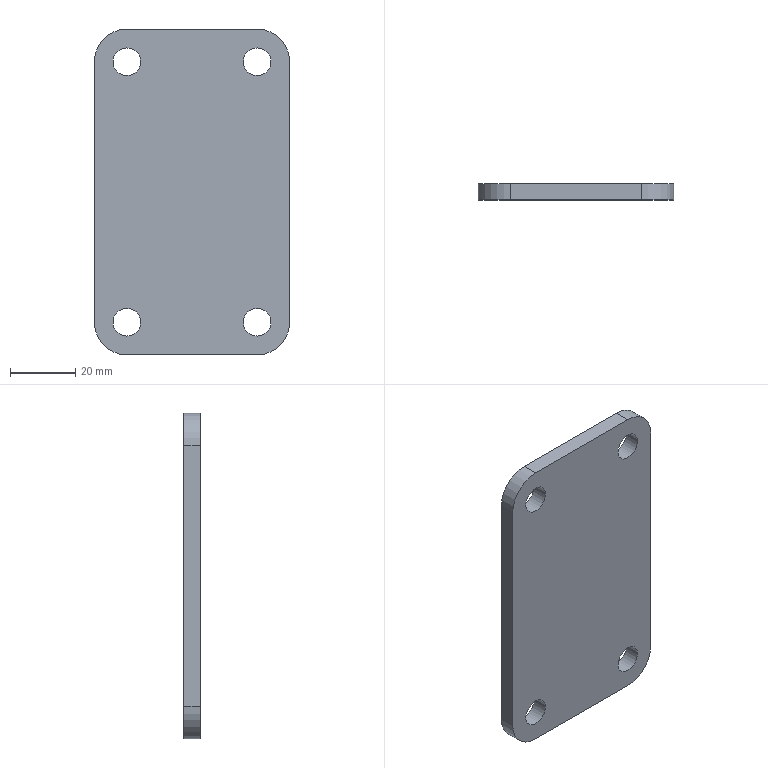Part | STEP file | JBJ-P-1004-04 | 1 solid | 14 faces | box 60 x 5 x 100 mm | volume 28436 mm3 | cylinder 8 | plane 6 | commonest cylinder face diameters 8.5 x4 20 x4
STEP:
#1=CARTESIAN_POINT('',(0.,5.,10.));
#2=VERTEX_POINT('',#1);
#3=CARTESIAN_POINT('',(0.,5.,90.));
#4=VERTEX_POINT('',#3);
#5=CARTESIAN_POINT('',(0.,5.,0.));
#6=DIRECTION('',(0.,0.,1.));
#7=VECTOR('',#6,1000.);
#8=LINE('',#5,#7);
#9=EDGE_CURVE('',#2,#4,#8,.T.);
#10=ORIENTED_EDGE('',*,*,#9,.F.);
#11=CARTESIAN_POINT('',(0.,0.,10.));
#12=VERTEX_POINT('',#11);
#13=CARTESIAN_POINT('',(0.,5.,10.));
#14=DIRECTION('',(0.,-1.,0.));
#15=VECTOR('',#14,1000.);
#16=LINE('',#13,#15);
#17=EDGE_CURVE('',#2,#12,#16,.T.);
#18=ORIENTED_EDGE('',*,*,#17,.T.);
#19=CARTESIAN_POINT('',(0.,0.,90.));
#20=VERTEX_POINT('',#19);
#21=CARTESIAN_POINT('',(0.,0.,0.));
#22=DIRECTION('',(0.,0.,1.));
#23=VECTOR('',#22,1000.);
#24=LINE('',#21,#23);
#25=EDGE_CURVE('',#12,#20,#24,.T.);
#26=ORIENTED_EDGE('',*,*,#25,.T.);
#27=CARTESIAN_POINT('',(0.,5.,90.));
#28=DIRECTION('',(0.,1.,0.));
#29=VECTOR('',#28,1000.);
#30=LINE('',#27,#29);
#31=EDGE_CURVE('',#20,#4,#30,.T.);
#32=ORIENTED_EDGE('',*,*,#31,.T.);
#33=EDGE_LOOP('',(#10,#18,#26,#32));
#34=FACE_OUTER_BOUND('',#33,.T.);
#35=CARTESIAN_POINT('',(0.,5.,0.));
#36=DIRECTION('',(1.,0.,0.));
#37=DIRECTION('',(0.,0.,-1.));
#38=AXIS2_PLACEMENT_3D('',#35,#36,#37);
#39=PLANE('',#38);
#40=ADVANCED_FACE('',(#34),#39,.F.);
#41=CARTESIAN_POINT('',(10.,0.,100.));
#42=VERTEX_POINT('',#41);
#43=CARTESIAN_POINT('',(50.,0.,100.));
#44=VERTEX_POINT('',#43);
#45=CARTESIAN_POINT('',(0.,0.,100.));
#46=DIRECTION('',(1.,0.,0.));
#47=VECTOR('',#46,1000.);
#48=LINE('',#45,#47);
#49=EDGE_CURVE('',#42,#44,#48,.T.);
#50=ORIENTED_EDGE('',*,*,#49,.T.);
#51=CARTESIAN_POINT('',(50.,5.,100.));
#52=VERTEX_POINT('',#51);
#53=CARTESIAN_POINT('',(50.,5.,100.));
#54=DIRECTION('',(0.,1.,0.));
#55=VECTOR('',#54,1000.);
#56=LINE('',#53,#55);
#57=EDGE_CURVE('',#44,#52,#56,.T.);
#58=ORIENTED_EDGE('',*,*,#57,.T.);
#59=CARTESIAN_POINT('',(10.,5.,100.));
#60=VERTEX_POINT('',#59);
#61=CARTESIAN_POINT('',(0.,5.,100.));
#62=DIRECTION('',(1.,0.,0.));
#63=VECTOR('',#62,1000.);
#64=LINE('',#61,#63);
#65=EDGE_CURVE('',#60,#52,#64,.T.);
#66=ORIENTED_EDGE('',*,*,#65,.F.);
#67=CARTESIAN_POINT('',(10.,5.,100.));
#68=DIRECTION('',(0.,-1.,0.));
#69=VECTOR('',#68,1000.);
#70=LINE('',#67,#69);
#71=EDGE_CURVE('',#60,#42,#70,.T.);
#72=ORIENTED_EDGE('',*,*,#71,.T.);
#73=EDGE_LOOP('',(#50,#58,#66,#72));
#74=FACE_OUTER_BOUND('',#73,.T.);
#75=CARTESIAN_POINT('',(0.,5.,100.));
#76=DIRECTION('',(0.,0.,-1.));
#77=DIRECTION('',(-1.,0.,0.));
#78=AXIS2_PLACEMENT_3D('',#75,#76,#77);
#79=PLANE('',#78);
#80=ADVANCED_FACE('',(#74),#79,.F.);
#81=CARTESIAN_POINT('',(60.,5.,90.));
#82=VERTEX_POINT('',#81);
#83=CARTESIAN_POINT('',(60.,5.,10.));
#84=VERTEX_POINT('',#83);
#85=CARTESIAN_POINT('',(60.,5.,0.));
#86=DIRECTION('',(0.,0.,-1.));
#87=VECTOR('',#86,1000.);
#88=LINE('',#85,#87);
#89=EDGE_CURVE('',#82,#84,#88,.T.);
#90=ORIENTED_EDGE('',*,*,#89,.F.);
#91=CARTESIAN_POINT('',(60.,0.,90.));
#92=VERTEX_POINT('',#91);
#93=CARTESIAN_POINT('',(60.,5.,90.));
#94=DIRECTION('',(0.,-1.,0.));
#95=VECTOR('',#94,1000.);
#96=LINE('',#93,#95);
#97=EDGE_CURVE('',#82,#92,#96,.T.);
#98=ORIENTED_EDGE('',*,*,#97,.T.);
#99=CARTESIAN_POINT('',(60.,0.,10.));
#100=VERTEX_POINT('',#99);
#101=CARTESIAN_POINT('',(60.,0.,0.));
#102=DIRECTION('',(0.,0.,-1.));
#103=VECTOR('',#102,1000.);
#104=LINE('',#101,#103);
#105=EDGE_CURVE('',#92,#100,#104,.T.);
#106=ORIENTED_EDGE('',*,*,#105,.T.);
#107=CARTESIAN_POINT('',(60.,5.,10.));
#108=DIRECTION('',(0.,1.,0.));
#109=VECTOR('',#108,1000.);
#110=LINE('',#107,#109);
#111=EDGE_CURVE('',#100,#84,#110,.T.);
#112=ORIENTED_EDGE('',*,*,#111,.T.);
#113=EDGE_LOOP('',(#90,#98,#106,#112));
#114=FACE_OUTER_BOUND('',#113,.T.);
#115=CARTESIAN_POINT('',(60.,5.,0.));
#116=DIRECTION('',(-1.,0.,0.));
#117=DIRECTION('',(0.,0.,1.));
#118=AXIS2_PLACEMENT_3D('',#115,#116,#117);
#119=PLANE('',#118);
#120=ADVANCED_FACE('',(#114),#119,.F.);
#121=CARTESIAN_POINT('',(50.,5.,0.));
#122=VERTEX_POINT('',#121);
#123=CARTESIAN_POINT('',(10.,5.,0.));
#124=VERTEX_POINT('',#123);
#125=CARTESIAN_POINT('',(0.,5.,0.));
#126=DIRECTION('',(-1.,0.,0.));
#127=VECTOR('',#126,1000.);
#128=LINE('',#125,#127);
#129=EDGE_CURVE('',#122,#124,#128,.T.);
#130=ORIENTED_EDGE('',*,*,#129,.F.);
#131=CARTESIAN_POINT('',(50.,0.,0.));
#132=VERTEX_POINT('',#131);
#133=CARTESIAN_POINT('',(50.,5.,0.));
#134=DIRECTION('',(0.,-1.,0.));
#135=VECTOR('',#134,1000.);
#136=LINE('',#133,#135);
#137=EDGE_CURVE('',#122,#132,#136,.T.);
#138=ORIENTED_EDGE('',*,*,#137,.T.);
#139=CARTESIAN_POINT('',(10.,0.,0.));
#140=VERTEX_POINT('',#139);
#141=CARTESIAN_POINT('',(0.,0.,0.));
#142=DIRECTION('',(-1.,0.,0.));
#143=VECTOR('',#142,1000.);
#144=LINE('',#141,#143);
#145=EDGE_CURVE('',#132,#140,#144,.T.);
#146=ORIENTED_EDGE('',*,*,#145,.T.);
#147=CARTESIAN_POINT('',(10.,5.,0.));
#148=DIRECTION('',(0.,1.,0.));
#149=VECTOR('',#148,1000.);
#150=LINE('',#147,#149);
#151=EDGE_CURVE('',#140,#124,#150,.T.);
#152=ORIENTED_EDGE('',*,*,#151,.T.);
#153=EDGE_LOOP('',(#130,#138,#146,#152));
#154=FACE_OUTER_BOUND('',#153,.T.);
#155=CARTESIAN_POINT('',(0.,5.,0.));
#156=DIRECTION('',(0.,0.,1.));
#157=DIRECTION('',(1.,0.,0.));
#158=AXIS2_PLACEMENT_3D('',#155,#156,#157);
#159=PLANE('',#158);
#160=ADVANCED_FACE('',(#154),#159,.F.);
#161=CARTESIAN_POINT('',(50.,5.,94.25));
#162=VERTEX_POINT('',#161);
#163=CARTESIAN_POINT('',(50.,5.,90.));
#164=DIRECTION('',(0.,1.,0.));
#165=DIRECTION('',(0.,0.,1.));
#166=AXIS2_PLACEMENT_3D('',#163,#164,#165);
#167=CIRCLE('',#166,4.25);
#168=EDGE_CURVE('',#162,#162,#167,.T.);
#169=ORIENTED_EDGE('',*,*,#168,.F.);
#170=EDGE_LOOP('',(#169));
#171=FACE_BOUND('',#170,.T.);
#172=CARTESIAN_POINT('',(10.,5.,94.25));
#173=VERTEX_POINT('',#172);
#174=CARTESIAN_POINT('',(10.,5.,90.));
#175=DIRECTION('',(0.,1.,0.));
#176=DIRECTION('',(0.,0.,1.));
#177=AXIS2_PLACEMENT_3D('',#174,#175,#176);
#178=CIRCLE('',#177,4.25);
#179=EDGE_CURVE('',#173,#173,#178,.T.);
#180=ORIENTED_EDGE('',*,*,#179,.F.);
#181=EDGE_LOOP('',(#180));
#182=FACE_BOUND('',#181,.T.);
#183=CARTESIAN_POINT('',(10.,5.,14.25));
#184=VERTEX_POINT('',#183);
#185=CARTESIAN_POINT('',(10.,5.,10.));
#186=DIRECTION('',(0.,1.,0.));
#187=DIRECTION('',(0.,0.,1.));
#188=AXIS2_PLACEMENT_3D('',#185,#186,#187);
#189=CIRCLE('',#188,4.25);
#190=EDGE_CURVE('',#184,#184,#189,.T.);
#191=ORIENTED_EDGE('',*,*,#190,.F.);
#192=EDGE_LOOP('',(#191));
#193=FACE_BOUND('',#192,.T.);
#194=CARTESIAN_POINT('',(50.,5.,14.25));
#195=VERTEX_POINT('',#194);
#196=CARTESIAN_POINT('',(50.,5.,10.));
#197=DIRECTION('',(0.,1.,0.));
#198=DIRECTION('',(0.,0.,1.));
#199=AXIS2_PLACEMENT_3D('',#196,#197,#198);
#200=CIRCLE('',#199,4.25);
#201=EDGE_CURVE('',#195,#195,#200,.T.);
#202=ORIENTED_EDGE('',*,*,#201,.F.);
#203=EDGE_LOOP('',(#202));
#204=FACE_BOUND('',#203,.T.);
#205=ORIENTED_EDGE('',*,*,#65,.T.);
#206=CARTESIAN_POINT('',(50.,5.,90.));
#207=DIRECTION('',(0.,1.,0.));
#208=DIRECTION('',(0.,0.,1.));
#209=AXIS2_PLACEMENT_3D('',#206,#207,#208);
#210=CIRCLE('',#209,10.);
#211=EDGE_CURVE('',#52,#82,#210,.T.);
#212=ORIENTED_EDGE('',*,*,#211,.T.);
#213=ORIENTED_EDGE('',*,*,#89,.T.);
#214=CARTESIAN_POINT('',(50.,5.,10.));
#215=DIRECTION('',(0.,1.,0.));
#216=DIRECTION('',(0.,0.,1.));
#217=AXIS2_PLACEMENT_3D('',#214,#215,#216);
#218=CIRCLE('',#217,10.);
#219=EDGE_CURVE('',#84,#122,#218,.T.);
#220=ORIENTED_EDGE('',*,*,#219,.T.);
#221=ORIENTED_EDGE('',*,*,#129,.T.);
#222=CARTESIAN_POINT('',(10.,5.,10.));
#223=DIRECTION('',(0.,1.,0.));
#224=DIRECTION('',(0.,0.,1.));
#225=AXIS2_PLACEMENT_3D('',#222,#223,#224);
#226=CIRCLE('',#225,10.);
#227=EDGE_CURVE('',#124,#2,#226,.T.);
#228=ORIENTED_EDGE('',*,*,#227,.T.);
#229=ORIENTED_EDGE('',*,*,#9,.T.);
#230=CARTESIAN_POINT('',(10.,5.,90.));
#231=DIRECTION('',(0.,1.,0.));
#232=DIRECTION('',(0.,0.,1.));
#233=AXIS2_PLACEMENT_3D('',#230,#231,#232);
#234=CIRCLE('',#233,10.);
#235=EDGE_CURVE('',#4,#60,#234,.T.);
#236=ORIENTED_EDGE('',*,*,#235,.T.);
#237=EDGE_LOOP('',(#205,#212,#213,#220,#221,#228,#229,#236));
#238=FACE_OUTER_BOUND('',#237,.T.);
#239=CARTESIAN_POINT('',(0.,5.,0.));
#240=DIRECTION('',(0.,1.,0.));
#241=DIRECTION('',(0.,0.,1.));
#242=AXIS2_PLACEMENT_3D('',#239,#240,#241);
#243=PLANE('',#242);
#244=ADVANCED_FACE('',(#171,#182,#193,#204,#238),#243,.T.);
#245=CARTESIAN_POINT('',(50.,0.,94.25));
#246=VERTEX_POINT('',#245);
#247=CARTESIAN_POINT('',(50.,0.,90.));
#248=DIRECTION('',(0.,1.,0.));
#249=DIRECTION('',(0.,0.,1.));
#250=AXIS2_PLACEMENT_3D('',#247,#248,#249);
#251=CIRCLE('',#250,4.25);
#252=EDGE_CURVE('',#246,#246,#251,.T.);
#253=ORIENTED_EDGE('',*,*,#252,.T.);
#254=EDGE_LOOP('',(#253));
#255=FACE_BOUND('',#254,.T.);
#256=CARTESIAN_POINT('',(10.,0.,94.25));
#257=VERTEX_POINT('',#256);
#258=CARTESIAN_POINT('',(10.,0.,90.));
#259=DIRECTION('',(0.,1.,0.));
#260=DIRECTION('',(0.,0.,1.));
#261=AXIS2_PLACEMENT_3D('',#258,#259,#260);
#262=CIRCLE('',#261,4.25);
#263=EDGE_CURVE('',#257,#257,#262,.T.);
#264=ORIENTED_EDGE('',*,*,#263,.T.);
#265=EDGE_LOOP('',(#264));
#266=FACE_BOUND('',#265,.T.);
#267=CARTESIAN_POINT('',(10.,0.,14.25));
#268=VERTEX_POINT('',#267);
#269=CARTESIAN_POINT('',(10.,0.,10.));
#270=DIRECTION('',(0.,1.,0.));
#271=DIRECTION('',(0.,0.,1.));
#272=AXIS2_PLACEMENT_3D('',#269,#270,#271);
#273=CIRCLE('',#272,4.25);
#274=EDGE_CURVE('',#268,#268,#273,.T.);
#275=ORIENTED_EDGE('',*,*,#274,.T.);
#276=EDGE_LOOP('',(#275));
#277=FACE_BOUND('',#276,.T.);
#278=CARTESIAN_POINT('',(50.,0.,14.25));
#279=VERTEX_POINT('',#278);
#280=CARTESIAN_POINT('',(50.,0.,10.));
#281=DIRECTION('',(0.,1.,0.));
#282=DIRECTION('',(0.,0.,1.));
#283=AXIS2_PLACEMENT_3D('',#280,#281,#282);
#284=CIRCLE('',#283,4.25);
#285=EDGE_CURVE('',#279,#279,#284,.T.);
#286=ORIENTED_EDGE('',*,*,#285,.T.);
#287=EDGE_LOOP('',(#286));
#288=FACE_BOUND('',#287,.T.);
#289=ORIENTED_EDGE('',*,*,#105,.F.);
#290=CARTESIAN_POINT('',(50.,0.,90.));
#291=DIRECTION('',(0.,-1.,0.));
#292=DIRECTION('',(0.,0.,1.));
#293=AXIS2_PLACEMENT_3D('',#290,#291,#292);
#294=CIRCLE('',#293,10.);
#295=EDGE_CURVE('',#92,#44,#294,.T.);
#296=ORIENTED_EDGE('',*,*,#295,.T.);
#297=ORIENTED_EDGE('',*,*,#49,.F.);
#298=CARTESIAN_POINT('',(10.,0.,90.));
#299=DIRECTION('',(0.,-1.,0.));
#300=DIRECTION('',(0.,0.,1.));
#301=AXIS2_PLACEMENT_3D('',#298,#299,#300);
#302=CIRCLE('',#301,10.);
#303=EDGE_CURVE('',#42,#20,#302,.T.);
#304=ORIENTED_EDGE('',*,*,#303,.T.);
#305=ORIENTED_EDGE('',*,*,#25,.F.);
#306=CARTESIAN_POINT('',(10.,0.,10.));
#307=DIRECTION('',(0.,-1.,0.));
#308=DIRECTION('',(0.,0.,1.));
#309=AXIS2_PLACEMENT_3D('',#306,#307,#308);
#310=CIRCLE('',#309,10.);
#311=EDGE_CURVE('',#12,#140,#310,.T.);
#312=ORIENTED_EDGE('',*,*,#311,.T.);
#313=ORIENTED_EDGE('',*,*,#145,.F.);
#314=CARTESIAN_POINT('',(50.,0.,10.));
#315=DIRECTION('',(0.,-1.,0.));
#316=DIRECTION('',(0.,0.,1.));
#317=AXIS2_PLACEMENT_3D('',#314,#315,#316);
#318=CIRCLE('',#317,10.);
#319=EDGE_CURVE('',#132,#100,#318,.T.);
#320=ORIENTED_EDGE('',*,*,#319,.T.);
#321=EDGE_LOOP('',(#289,#296,#297,#304,#305,#312,#313,#320));
#322=FACE_OUTER_BOUND('',#321,.T.);
#323=CARTESIAN_POINT('',(0.,0.,0.));
#324=DIRECTION('',(0.,1.,0.));
#325=DIRECTION('',(0.,0.,1.));
#326=AXIS2_PLACEMENT_3D('',#323,#324,#325);
#327=PLANE('',#326);
#328=ADVANCED_FACE('',(#255,#266,#277,#288,#322),#327,.F.);
#329=ORIENTED_EDGE('',*,*,#211,.F.);
#330=ORIENTED_EDGE('',*,*,#57,.F.);
#331=ORIENTED_EDGE('',*,*,#295,.F.);
#332=ORIENTED_EDGE('',*,*,#97,.F.);
#333=EDGE_LOOP('',(#329,#330,#331,#332));
#334=FACE_OUTER_BOUND('',#333,.T.);
#335=CARTESIAN_POINT('',(50.,5.,90.));
#336=DIRECTION('',(0.,-1.,0.));
#337=DIRECTION('',(0.,0.,-1.));
#338=AXIS2_PLACEMENT_3D('',#335,#336,#337);
#339=CYLINDRICAL_SURFACE('',#338,10.);
#340=ADVANCED_FACE('',(#334),#339,.T.);
#341=ORIENTED_EDGE('',*,*,#219,.F.);
#342=ORIENTED_EDGE('',*,*,#111,.F.);
#343=ORIENTED_EDGE('',*,*,#319,.F.);
#344=ORIENTED_EDGE('',*,*,#137,.F.);
#345=EDGE_LOOP('',(#341,#342,#343,#344));
#346=FACE_OUTER_BOUND('',#345,.T.);
#347=CARTESIAN_POINT('',(50.,5.,10.));
#348=DIRECTION('',(0.,-1.,0.));
#349=DIRECTION('',(0.,0.,-1.));
#350=AXIS2_PLACEMENT_3D('',#347,#348,#349);
#351=CYLINDRICAL_SURFACE('',#350,10.);
#352=ADVANCED_FACE('',(#346),#351,.T.);
#353=ORIENTED_EDGE('',*,*,#227,.F.);
#354=ORIENTED_EDGE('',*,*,#151,.F.);
#355=ORIENTED_EDGE('',*,*,#311,.F.);
#356=ORIENTED_EDGE('',*,*,#17,.F.);
#357=EDGE_LOOP('',(#353,#354,#355,#356));
#358=FACE_OUTER_BOUND('',#357,.T.);
#359=CARTESIAN_POINT('',(10.,5.,10.));
#360=DIRECTION('',(0.,-1.,0.));
#361=DIRECTION('',(0.,0.,-1.));
#362=AXIS2_PLACEMENT_3D('',#359,#360,#361);
#363=CYLINDRICAL_SURFACE('',#362,10.);
#364=ADVANCED_FACE('',(#358),#363,.T.);
#365=ORIENTED_EDGE('',*,*,#235,.F.);
#366=ORIENTED_EDGE('',*,*,#31,.F.);
#367=ORIENTED_EDGE('',*,*,#303,.F.);
#368=ORIENTED_EDGE('',*,*,#71,.F.);
#369=EDGE_LOOP('',(#365,#366,#367,#368));
#370=FACE_OUTER_BOUND('',#369,.T.);
#371=CARTESIAN_POINT('',(10.,5.,90.));
#372=DIRECTION('',(0.,-1.,0.));
#373=DIRECTION('',(0.,0.,-1.));
#374=AXIS2_PLACEMENT_3D('',#371,#372,#373);
#375=CYLINDRICAL_SURFACE('',#374,10.);
#376=ADVANCED_FACE('',(#370),#375,.T.);
#377=ORIENTED_EDGE('',*,*,#201,.T.);
#378=EDGE_LOOP('',(#377));
#379=FACE_OUTER_BOUND('',#378,.T.);
#380=ORIENTED_EDGE('',*,*,#285,.F.);
#381=EDGE_LOOP('',(#380));
#382=FACE_OUTER_BOUND('',#381,.T.);
#383=CARTESIAN_POINT('',(50.,5.,10.));
#384=DIRECTION('',(0.,1.,0.));
#385=DIRECTION('',(0.,0.,1.));
#386=AXIS2_PLACEMENT_3D('',#383,#384,#385);
#387=CYLINDRICAL_SURFACE('',#386,4.25);
#388=ADVANCED_FACE('',(#379,#382),#387,.F.);
#389=ORIENTED_EDGE('',*,*,#190,.T.);
#390=EDGE_LOOP('',(#389));
#391=FACE_OUTER_BOUND('',#390,.T.);
#392=ORIENTED_EDGE('',*,*,#274,.F.);
#393=EDGE_LOOP('',(#392));
#394=FACE_OUTER_BOUND('',#393,.T.);
#395=CARTESIAN_POINT('',(10.,5.,10.));
#396=DIRECTION('',(0.,1.,0.));
#397=DIRECTION('',(0.,0.,1.));
#398=AXIS2_PLACEMENT_3D('',#395,#396,#397);
#399=CYLINDRICAL_SURFACE('',#398,4.25);
#400=ADVANCED_FACE('',(#391,#394),#399,.F.);
#401=ORIENTED_EDGE('',*,*,#179,.T.);
#402=EDGE_LOOP('',(#401));
#403=FACE_OUTER_BOUND('',#402,.T.);
#404=ORIENTED_EDGE('',*,*,#263,.F.);
#405=EDGE_LOOP('',(#404));
#406=FACE_OUTER_BOUND('',#405,.T.);
#407=CARTESIAN_POINT('',(10.,5.,90.));
#408=DIRECTION('',(0.,1.,0.));
#409=DIRECTION('',(0.,0.,1.));
#410=AXIS2_PLACEMENT_3D('',#407,#408,#409);
#411=CYLINDRICAL_SURFACE('',#410,4.25);
#412=ADVANCED_FACE('',(#403,#406),#411,.F.);
#413=ORIENTED_EDGE('',*,*,#168,.T.);
#414=EDGE_LOOP('',(#413));
#415=FACE_OUTER_BOUND('',#414,.T.);
#416=ORIENTED_EDGE('',*,*,#252,.F.);
#417=EDGE_LOOP('',(#416));
#418=FACE_OUTER_BOUND('',#417,.T.);
#419=CARTESIAN_POINT('',(50.,5.,90.));
#420=DIRECTION('',(0.,1.,0.));
#421=DIRECTION('',(0.,0.,1.));
#422=AXIS2_PLACEMENT_3D('',#419,#420,#421);
#423=CYLINDRICAL_SURFACE('',#422,4.25);
#424=ADVANCED_FACE('',(#415,#418),#423,.F.);
#425=CLOSED_SHELL('',(#40,#80,#120,#160,#244,#328,#340,#352,#364,#376,#388,#400,#412,#424));
#426=MANIFOLD_SOLID_BREP('',#425);
#427=CARTESIAN_POINT('',(0.,0.,0.));
#428=DIRECTION('',(0.,0.,1.));
#429=DIRECTION('',(1.,0.,0.));
#430=AXIS2_PLACEMENT_3D('',#427,#428,#429);
#431=(LENGTH_UNIT()NAMED_UNIT(*)SI_UNIT(.MILLI.,.METRE.));
#432=UNCERTAINTY_MEASURE_WITH_UNIT(LENGTH_MEASURE(0.00001),#431,'','');
#433=(NAMED_UNIT(*)PLANE_ANGLE_UNIT()SI_UNIT($,.RADIAN.));
#434=(NAMED_UNIT(*)SI_UNIT($,.STERADIAN.)SOLID_ANGLE_UNIT());
#435=(GEOMETRIC_REPRESENTATION_CONTEXT(3)GLOBAL_UNCERTAINTY_ASSIGNED_CONTEXT((#432))GLOBAL_UNIT_ASSIGNED_CONTEXT((#431,#433,#434))REPRESENTATION_CONTEXT('',''));
#436=ADVANCED_BREP_SHAPE_REPRESENTATION('',(#426,#430),#435);